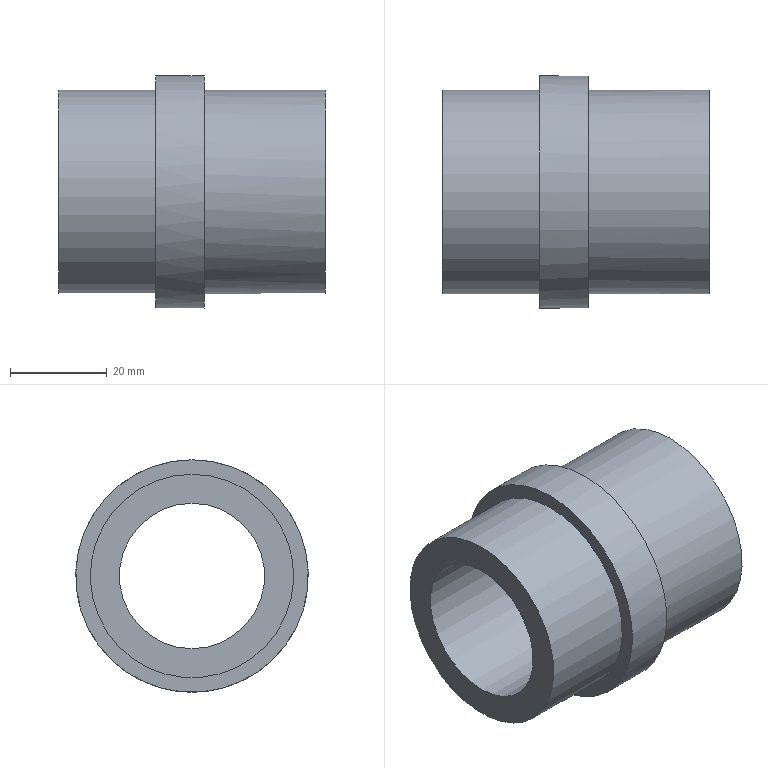Part | STEP file | solid 74 | 1 solid | 8 faces | box 55 x 48 x 48 mm | volume 41563 mm3 | plane 4 | cylinder 4 | commonest cylinder face diameters 42 x2 30 x1 48 x1